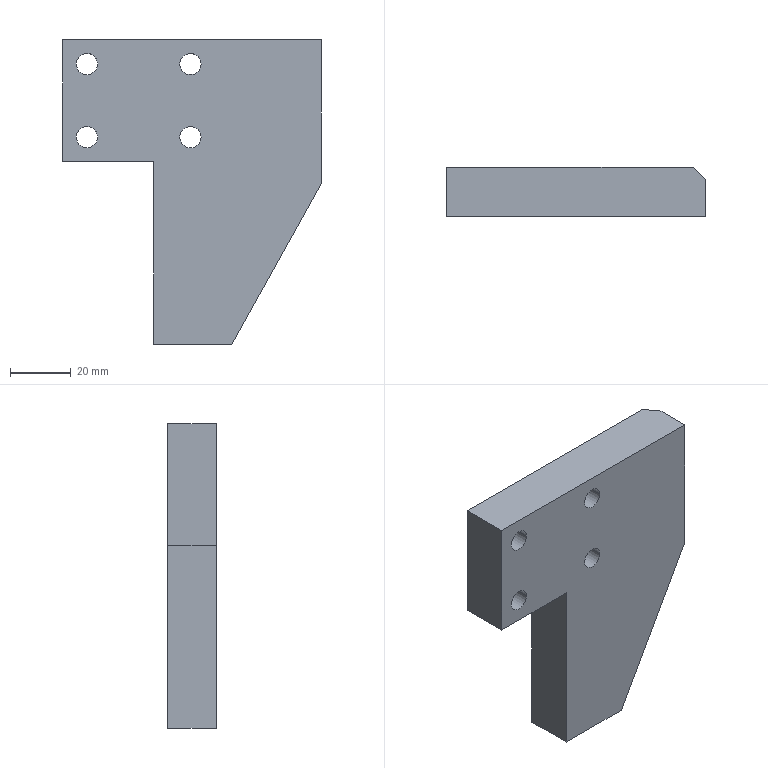Part | STEP file | Positioning_id2142_x_t | 1 solid | 19 faces | box 85 x 16 x 100 mm | volume 91411 mm3 | plane 11 | cylinder 8 | commonest cylinder face diameters 7 x8